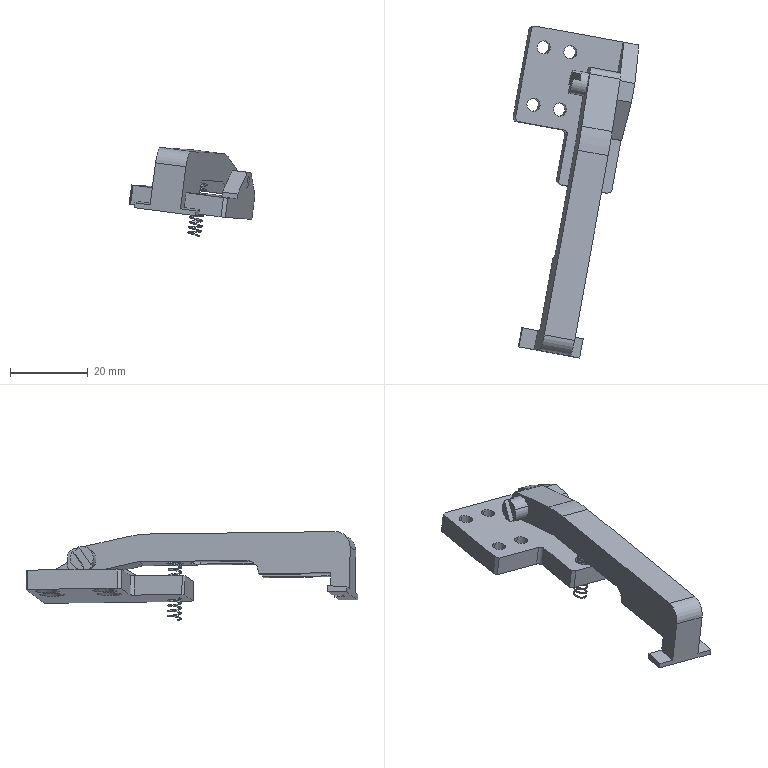Part | NX | features BREP 5 | 4 solids | 122 faces | box 32.394 x 85.445 x 22.853 mm | volume 8438 mm3 | plane 55 | cylinder 55 | cone 8 | spline 4 | commonest cylinder face diameters 3 x18 6 x9 3.4 x8 4.5 x7 2.5 x4 5 x4